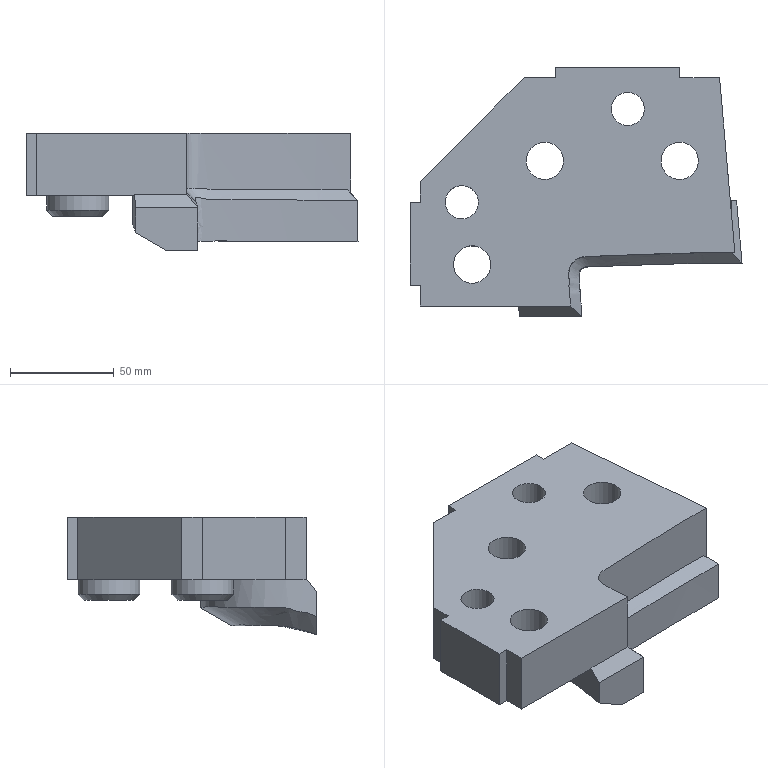Part | NX | features solid 2 | 1 solid | 43 faces | box 160.024 x 120 x 56.49 mm | volume 450764 mm3 | plane 25 | cylinder 10 | spline 6 | cone 2 | commonest cylinder face diameters 18 x3 26 x3 16 x2 30 x2